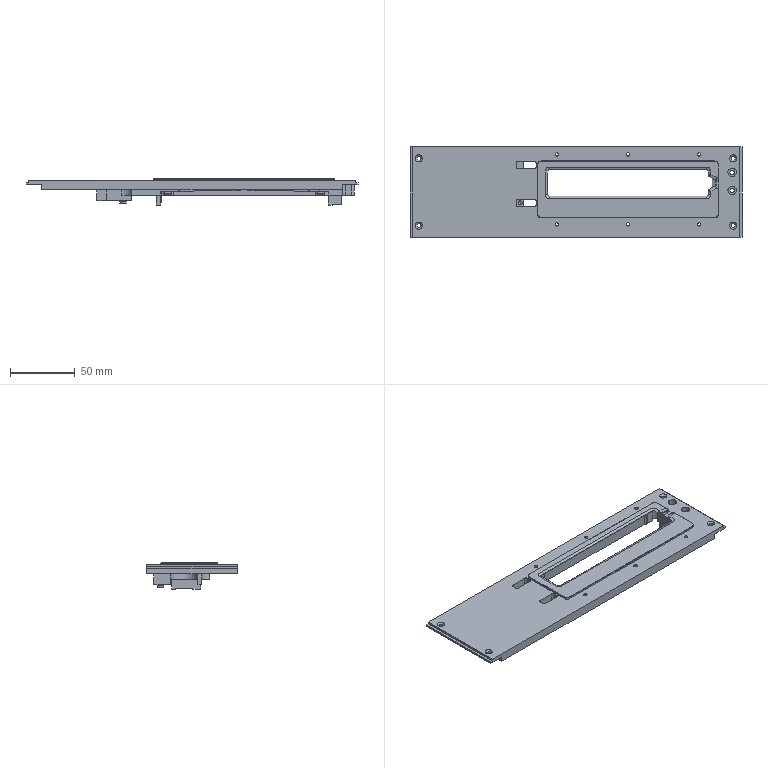NC program | NX | posted with a generic post | part box 256.6 x 70.3 x 20.422 mm
Lines 1 to 60 of 23702:
N10 G17 G21 G94 G90
(FLOOR_WALL_COPY , TOOL : D63)
N12 T01 M6
N14 G54
N16 G17 G0 G90 X-162.8 Y35.147 S6500 M3
N18 G43 Z30. H1
N20 Z7.
N22 G94 G1 Z4. F1250.
N24 X-159.8
N26 X159.8
N28 Y-9.95
N30 X-159.8
N32 X-162.8
N34 Z7.
N36 G0 Z30.
N38 Y35.147
N40 Z6.
N42 G1 Z3.
N44 X-159.8
N46 X159.8
N48 Y-9.95
N50 X-159.8
N52 X-162.8
N54 Z6.
N56 G0 Z30.
N58 Y35.147
N60 Z5.
N62 G1 Z2.
N64 X-159.8
N66 X159.8
N68 Y-9.95
N70 X-159.8
N72 X-162.8
N74 Z5.
N76 G0 Z30.
N78 Y35.147
N80 Z4.
N82 G1 Z1.
N84 X-159.8
N86 X159.8
N88 Y-9.95
N90 X-159.8
N92 X-162.8
N94 Z4.
N96 G0 Z30.
N98 Y35.147
N100 Z3.
N102 G1 Z0.
N104 X-159.8
N106 X159.8
N108 Y-9.95
N110 X-159.8
N112 X-162.8
N114 Z3.
N116 G0 Z30.
N118 M5